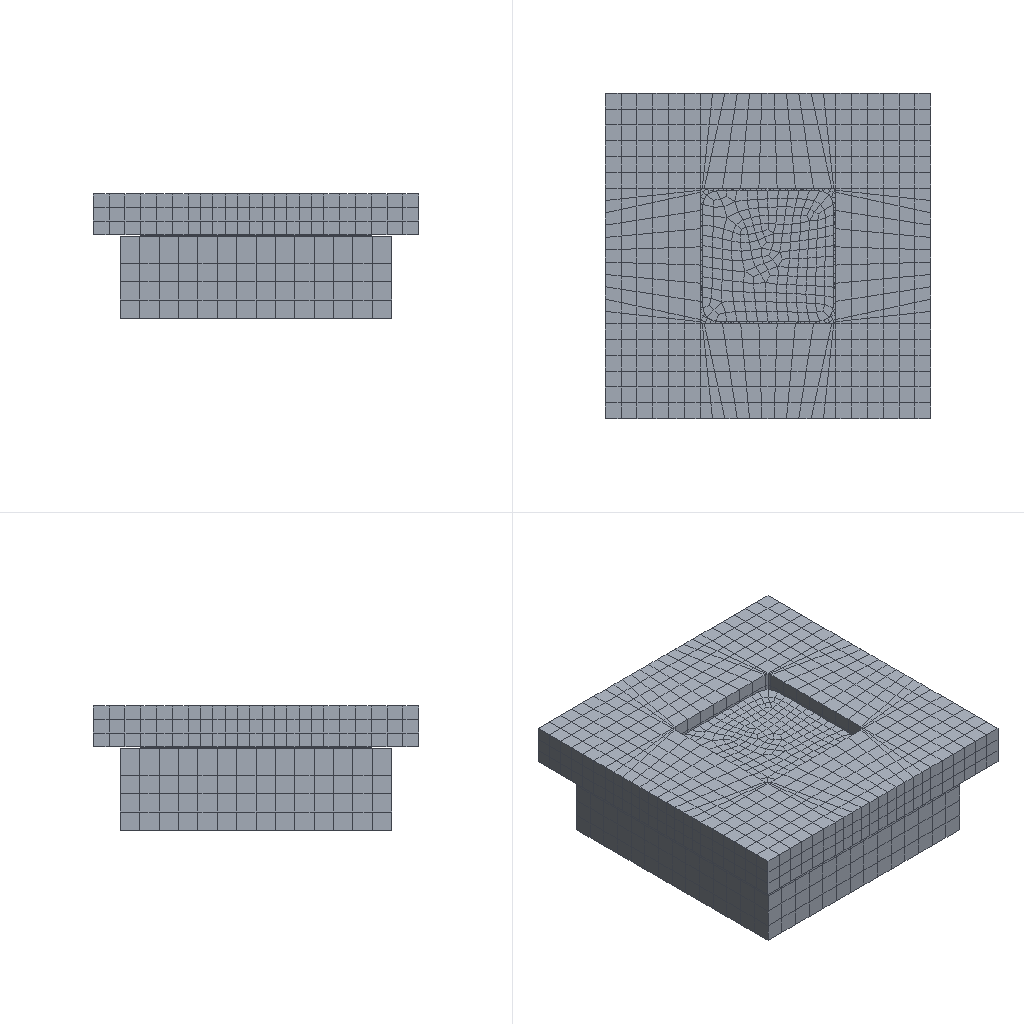Simulation study | abaqus
Set-up summary:
category,name,step,type,value,unit,region
solver,abaqus
solver,version,,,Abaqus/Explicit 2024
units,not stated in the deck,,not stated
analysis,deck,,transient,transient
load_step,load,load,transient,nlgeom=True
load_step,Step-1,Step-1,transient,nlgeom=True
contact,interactions,,,general=1 pairs=0 ties=0
load_step,requested,,,2
mesh,nodes,,,6159
mesh,elements,,,4703
element_type,S3,,shell,48
element_type,S4R,,shell,1764
element_type,C3D8R,,solid,2891
load,load commands in deck,,count,2
bc,support commands in deck,,count,13
material,MATERIAL-1,,in results
check,setup vs results,,match,"per instance, exact: element labels, types and connectivity; labels of the nodes the elements use; coordinates of those nodes at SINGLE_PRECISION in 4 of 4 instance(s)"
Abaqus input file, long lists of numbers shortened:
*Heading
** Job name: Job-1 Model name: Model-1
** Generated by: Abaqus/CAE 2024
*Preprint, echo=NO, model=NO, history=NO, contact=NO
**
** PARTS
**
*Part, name=Part-5
*Node
      1,   42.08,   5.959,           0.
      2,   40.829,   11.8,           0.
** (1854 more lines like these left out)
*Element, type=S3
 1, 1552,  714,  743
 2, 1650,  890,  167
** (46 more lines like these left out)
*Element, type=S4R
  49,  501,  392,   10,  494
  50,  389,  223,  499,    8
** (1762 more lines like these left out)
*Nset, nset=_PickedSet2, internal, generate
    1,  1856,     1
*Elset, elset=_PickedSet2, internal, generate
    1,  1812,     1
** Section: Section-1
*Shell Section, elset=_PickedSet2, material=Material-1
0.8, 5
*End Part
**
*Part, name=aomo
*Node
      1,         -25.,         -20.,          20.
      2,         -25.,          20.,          20.
** (1453 more lines like these left out)
*Element, type=C3D8R
  1,  335,  299,    1,  291, 1074, 1038,  131, 1030
  2,  329,   75,   74,  301, 1068,  618,  619, 1040
** (1020 more lines like these left out)
*Nset, nset=_PickedSet2, internal, generate
    1,  1455,     1
*Elset, elset=_PickedSet2, internal, generate
    1,  1022,     1
** Section: Section-2
*Solid Section, elset=_PickedSet2, material=Material-1
,
*End Part
**
*Part, name=tumo
*Node
      1,  -19.12,   24.12,           0.
      2,   19.12,   24.12,           0.
** (910 more lines like these left out)
*Element, type=C3D8R
  1,  52,  35,  34,  49, 280, 263, 262, 277
  2,  66,   4,   3,  50, 294, 232, 231, 278
** (607 more lines like these left out)
*Nset, nset=_PickedSet2, internal, generate
   1,  912,    1
*Elset, elset=_PickedSet2, internal, generate
   1,  609,    1
** Section: Section-2
*Solid Section, elset=_PickedSet2, material=Material-1
,
*End Part
**
*Part, name=yabianquan
*Node
      1,          25.,         -25.,           0.
      2,          25.,         -25.,          15.
** (1934 more lines like these left out)
*Element, type=C3D8R
  1,   86,  479, 1329,  429,    1,   49,  409,   62
  2,  479,  480, 1330, 1329,   49,   50,  410,  409
** (1258 more lines like these left out)
*Nset, nset=_PickedSet2, internal, generate
    1,  1936,     1
*Elset, elset=_PickedSet2, internal, generate
    1,  1260,     1
** Section: Section-2
*Solid Section, elset=_PickedSet2, material=Material-1
,
*End Part
**
**
** ASSEMBLY
**
*Assembly, name=Assembly
**
*Instance, name=aomo-1, part=aomo
          0.,           0.,         -30.
*End Instance
**
*Instance, name=tumo-1, part=tumo
          0.,           0.,          0.8
*End Instance
**
*Instance, name=yabianquan-1, part=yabianquan
          0.,           0.,          0.8
*End Instance
**
*Instance, name=Part-5-1, part=Part-5
          0.,           0.,          0.4
*End Instance
**
*Node
      1,          60.,         -60.,   15.8
*Node
      2,           0.,           0.,   10.8
*Node
      3,          50.,         -50.,         -30.
*Nset, nset=_PickedSet16, internal
 3,
*Nset, nset=_PickedSet17, internal, instance=aomo-1, generate
    1,  1455,     1
*Elset, elset=_PickedSet17, internal, instance=aomo-1, generate
    1,  1022,     1
*Nset, nset=_PickedSet18, internal
 1,
*Nset, nset=_PickedSet20, internal
 2,
*Nset, nset=_PickedSet21, internal, instance=tumo-1, generate
   1,  912,    1
*Elset, elset=_PickedSet21, internal, instance=tumo-1, generate
   1,  609,    1
*Nset, nset=_PickedSet23, internal
 2,
*Nset, nset=_PickedSet24, internal
 3,
*Nset, nset=_PickedSet25, internal
 1,
*Nset, nset=_PickedSet26, internal
 1,
*Nset, nset=_PickedSet27, internal, instance=yabianquan-1, generate
    1,  1936,     1
*Elset, elset=_PickedSet27, internal, instance=yabianquan-1, generate
    1,  1260,     1
** Constraint: Constraint-1
*Rigid Body, ref node=_PickedSet16, elset=_PickedSet17
** Constraint: Constraint-2
*Rigid Body, ref node=_PickedSet18, elset=_PickedSet27
** Constraint: Constraint-3
*Rigid Body, ref node=_PickedSet20, elset=_PickedSet21
*End Assembly
*Amplitude, name=Amp-1
             0.,              0.,             0.3,              1.
*Amplitude, name=Amp-2
             0.,              0.,            0.01,              1.
**
** MATERIALS
**
*Material, name=Material-1
*Density
 2.68e-09,
*Elastic
70000., 0.33
*Plastic
120.,   0.
180., 0.05
220., 0.15
235., 0.27
**
** INTERACTION PROPERTIES
**
*Surface Interaction, name=IntProp-1
*Friction
 0.1,
*Surface Behavior, pressure-overclosure=HARD
**
** BOUNDARY CONDITIONS
**
** Name: BC-1 Type: Symmetry/Antisymmetry/Encastre
*Boundary
_PickedSet24, ENCASTRE
** Name: BC-3 Type: Displacement/Rotation
*Boundary
_PickedSet25, 1, 1
_PickedSet25, 2, 2
_PickedSet25, 4, 4
_PickedSet25, 5, 5
_PickedSet25, 6, 6
**
** INTERACTIONS
**
** Interaction: Int-1
*Contact, op=NEW
*Contact Inclusions, ALL EXTERIOR
*Contact Property Assignment
 ,  , IntProp-1
** ----------------------------------------------------------------
**
** STEP: load
**
*Step, name=load, nlgeom=YES
*Dynamic, Explicit
, 0.01
*Bulk Viscosity
0.06, 1.2
** Mass Scaling: Semi-Automatic
**               Whole Model
*Fixed Mass Scaling, factor=1000.
**
** LOADS
**
** Name: Load-1   Type: Concentrated force
*Cload, amplitude=Amp-2
_PickedSet26, 3, -200.
**
** OUTPUT REQUESTS
**
*Restart, write, number interval=1, time marks=NO
**
** FIELD OUTPUT: F-Output-1
**
*Output, field
*Node Output
A, RF, U, V
*Element Output, directions=YES
EVF, LE, PE, PEEQ, PEEQVAVG, PEVAVG, S, STH, SVAVG
*Contact Output
CSTRESS,
**
** HISTORY OUTPUT: H-Output-1
**
*Output, history, variable=PRESELECT
*End Step
** ----------------------------------------------------------------
**
** STEP: Step-1
**
*Step, name=Step-1, nlgeom=YES
*Dynamic, Explicit
, 0.3
*Bulk Viscosity
0.06, 1.2
** Mass Scaling: Semi-Automatic
**               Whole Model
*Fixed Mass Scaling, factor=100.
**
** BOUNDARY CONDITIONS
**
** Name: BC-2 Type: Displacement/Rotation
*Boundary, amplitude=Amp-1
_PickedSet23, 1, 1
_PickedSet23, 2, 2
_PickedSet23, 3, 3, -10.
_PickedSet23, 4, 4
_PickedSet23, 5, 5
_PickedSet23, 6, 6
** Name: BC-3 Type: Displacement/Rotation
*Boundary
_PickedSet25, 3, 3
**
** OUTPUT REQUESTS
**
*Restart, write, number interval=1, time marks=NO
**
** FIELD OUTPUT: F-Output-1
**
*Output, field
*Node Output
A, RF, U, V
*Element Output, directions=YES
EVF, LE, PE, PEEQ, PEEQVAVG, PEVAVG, S, STH, SVAVG
*Contact Output
CSTRESS,
**
** HISTORY OUTPUT: H-Output-1
**
*Output, history, variable=PRESELECT
*End Step
Results summary:
result,step,load,completed,increments=2491 time=0.01/0.01
result,step,Step-1,completed,increments=383227 time=0.3/0.3
result,analysis,,,transient
result,last_loadstep,,,2
result,analysis steps,,count,2
result,primary field,,,"U, UR"
result,reaction total,,FX,57.719,model units
result,reaction total,,FY,20.63,model units
result,reaction total,,FZ,120.078,model units